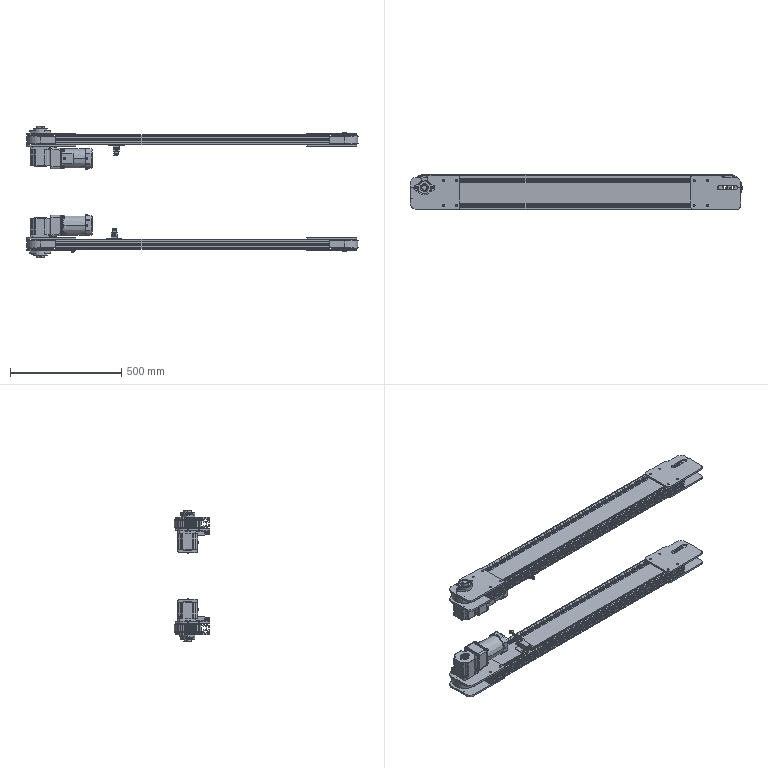Part | SolidWorks | 43 solids | 5727 faces | volume 11792712 mm3 | plane 2941 | cylinder 2072 | torus 302 | cone 196 | spline 168 | sphere 48 | commonest cylinder face diameters 1.6 x680 2 x220 112.75 x144 4 x88 8.5 x80 10 x60